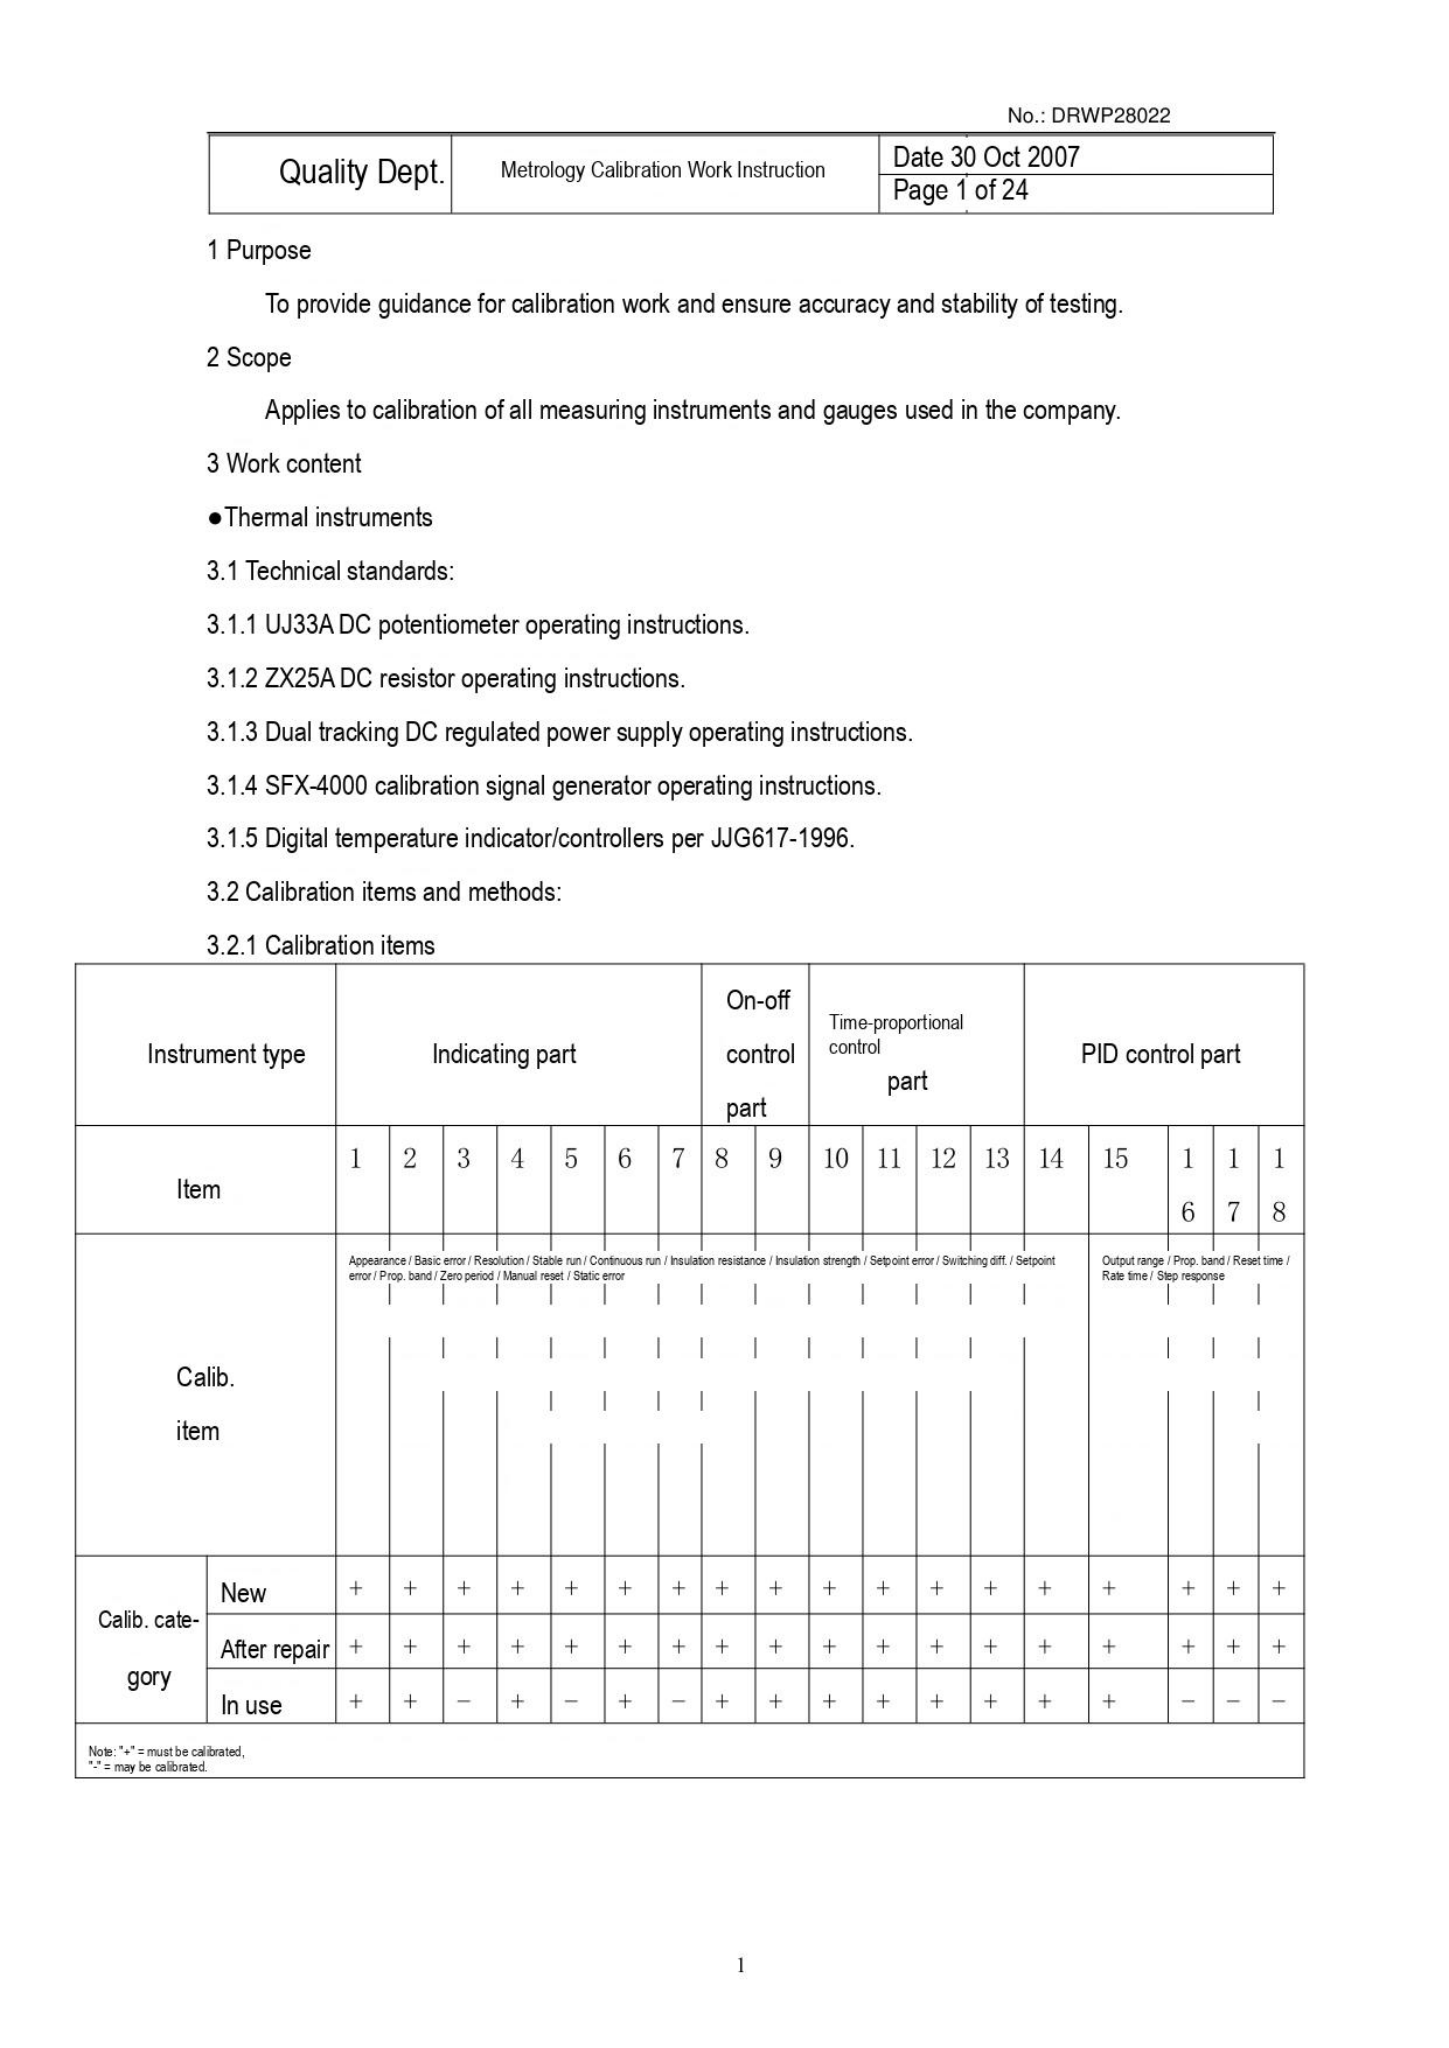No.: DRWP28022

| Quality Dept. | Metrology Calibration Work Instruction | Date 30 Oct 2007 |
|---|---|---|
| | | Page 1 of 24 |

1 Purpose

To provide guidance for calibration work and ensure accuracy and stability of testing.

2 Scope

Applies to calibration of all measuring instruments and gauges used in the company.

3 Work content

●Thermal instruments

3.1 Technical standards:

3.1.1 UJ33A DC potentiometer operating instructions.

3.1.2 ZX25A DC resistor operating instructions.

3.1.3 Dual tracking DC regulated power supply operating instructions.

3.1.4 SFX-4000 calibration signal generator operating instructions.

3.1.5 Digital temperature indicator/controllers per JJG617-1996.

3.2 Calibration items and methods:

3.2.1 Calibration items

| Instrument type | | Indicating part | | | | | | | On-off control part | | Time-proportional control part | | | | PID control part | | | | |
|---|---|---|---|---|---|---|---|---|---|---|---|---|---|---|---|---|---|---|---|
| Item | | 1 | 2 | 3 | 4 | 5 | 6 | 7 | 8 | 9 | 10 | 11 | 12 | 13 | 14 | 15 | 16 | 17 | 18 |
| Calib. item | | Appearance / Basic error / Resolution / Stable run / Continuous run / Insulation resistance / Insulation strength / Setpoint error / Switching diff. / Setpoint error / Prop. band / Zero period / Manual reset / Static error | | | | | | | | | | | | | | Output range / Prop. band / Reset time / Rate time / Step response | | | |
| Calib. category | New | + | + | + | + | + | + | + | + | + | + | + | + | + | + | + | + | + | + |
| | After repair | + | + | + | + | + | + | + | + | + | + | + | + | + | + | + | + | + | + |
| | In use | + | + | − | + | − | + | − | + | + | + | + | + | + | + | + | − | − | − |
| Note: "+" = must be calibrated, "-" = may be calibrated. | | | | | | | | | | | | | | | | | | | |

1
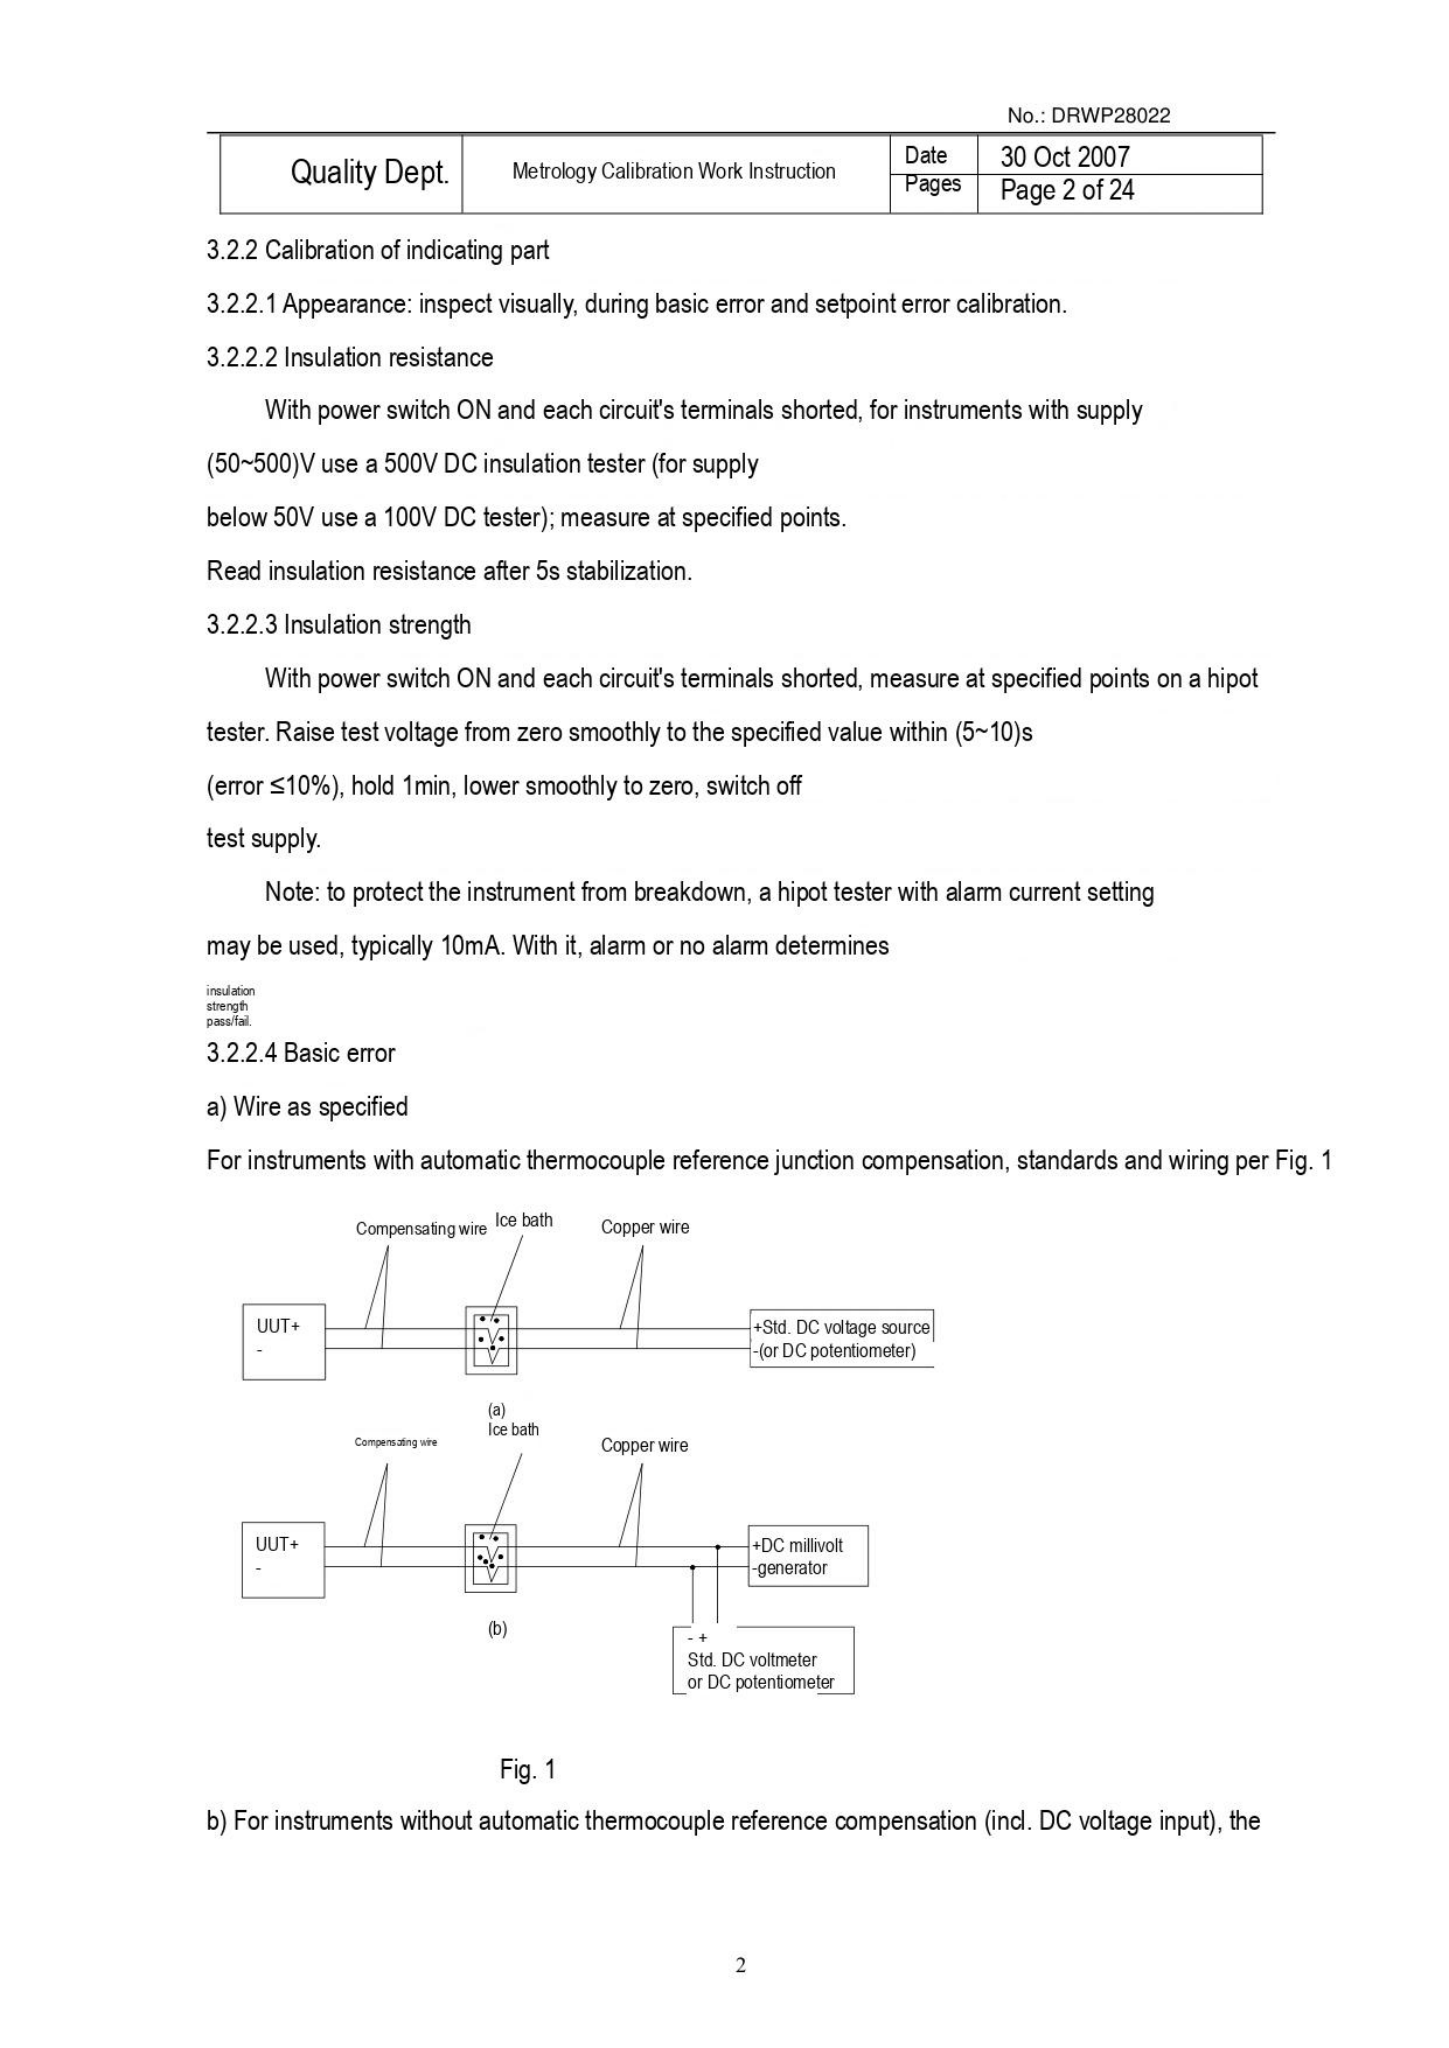No.: DRWP28022

| Quality Dept. | Metrology Calibration Work Instruction | Date | 30 Oct 2007 |
|---|---|---|---|
| | | Pages | Page 2 of 24 |

3.2.2 Calibration of indicating part

3.2.2.1 Appearance: inspect visually, during basic error and setpoint error calibration.

3.2.2.2 Insulation resistance

With power switch ON and each circuit's terminals shorted, for instruments with supply (50~500)V use a 500V DC insulation tester (for supply below 50V use a 100V DC tester); measure at specified points. Read insulation resistance after 5s stabilization.

3.2.2.3 Insulation strength

With power switch ON and each circuit's terminals shorted, measure at specified points on a hipot tester. Raise test voltage from zero smoothly to the specified value within (5~10)s (error ≤10%), hold 1min, lower smoothly to zero, switch off test supply.

Note: to protect the instrument from breakdown, a hipot tester with alarm current setting may be used, typically 10mA. With it, alarm or no alarm determines insulation strength pass/fail.

3.2.2.4 Basic error

a) Wire as specified

For instruments with automatic thermocouple reference junction compensation, standards and wiring per Fig. 1

Compensating wire Ice bath Copper wire

UUT+
-

+Std. DC voltage source
-(or DC potentiometer)

(a)

Ice bath

Compensating wire

Copper wire

UUT+
-

+DC millivolt
-generator

- +
Std. DC voltmeter
or DC potentiometer

(b)

Fig. 1

b) For instruments without automatic thermocouple reference compensation (incl. DC voltage input), the

2
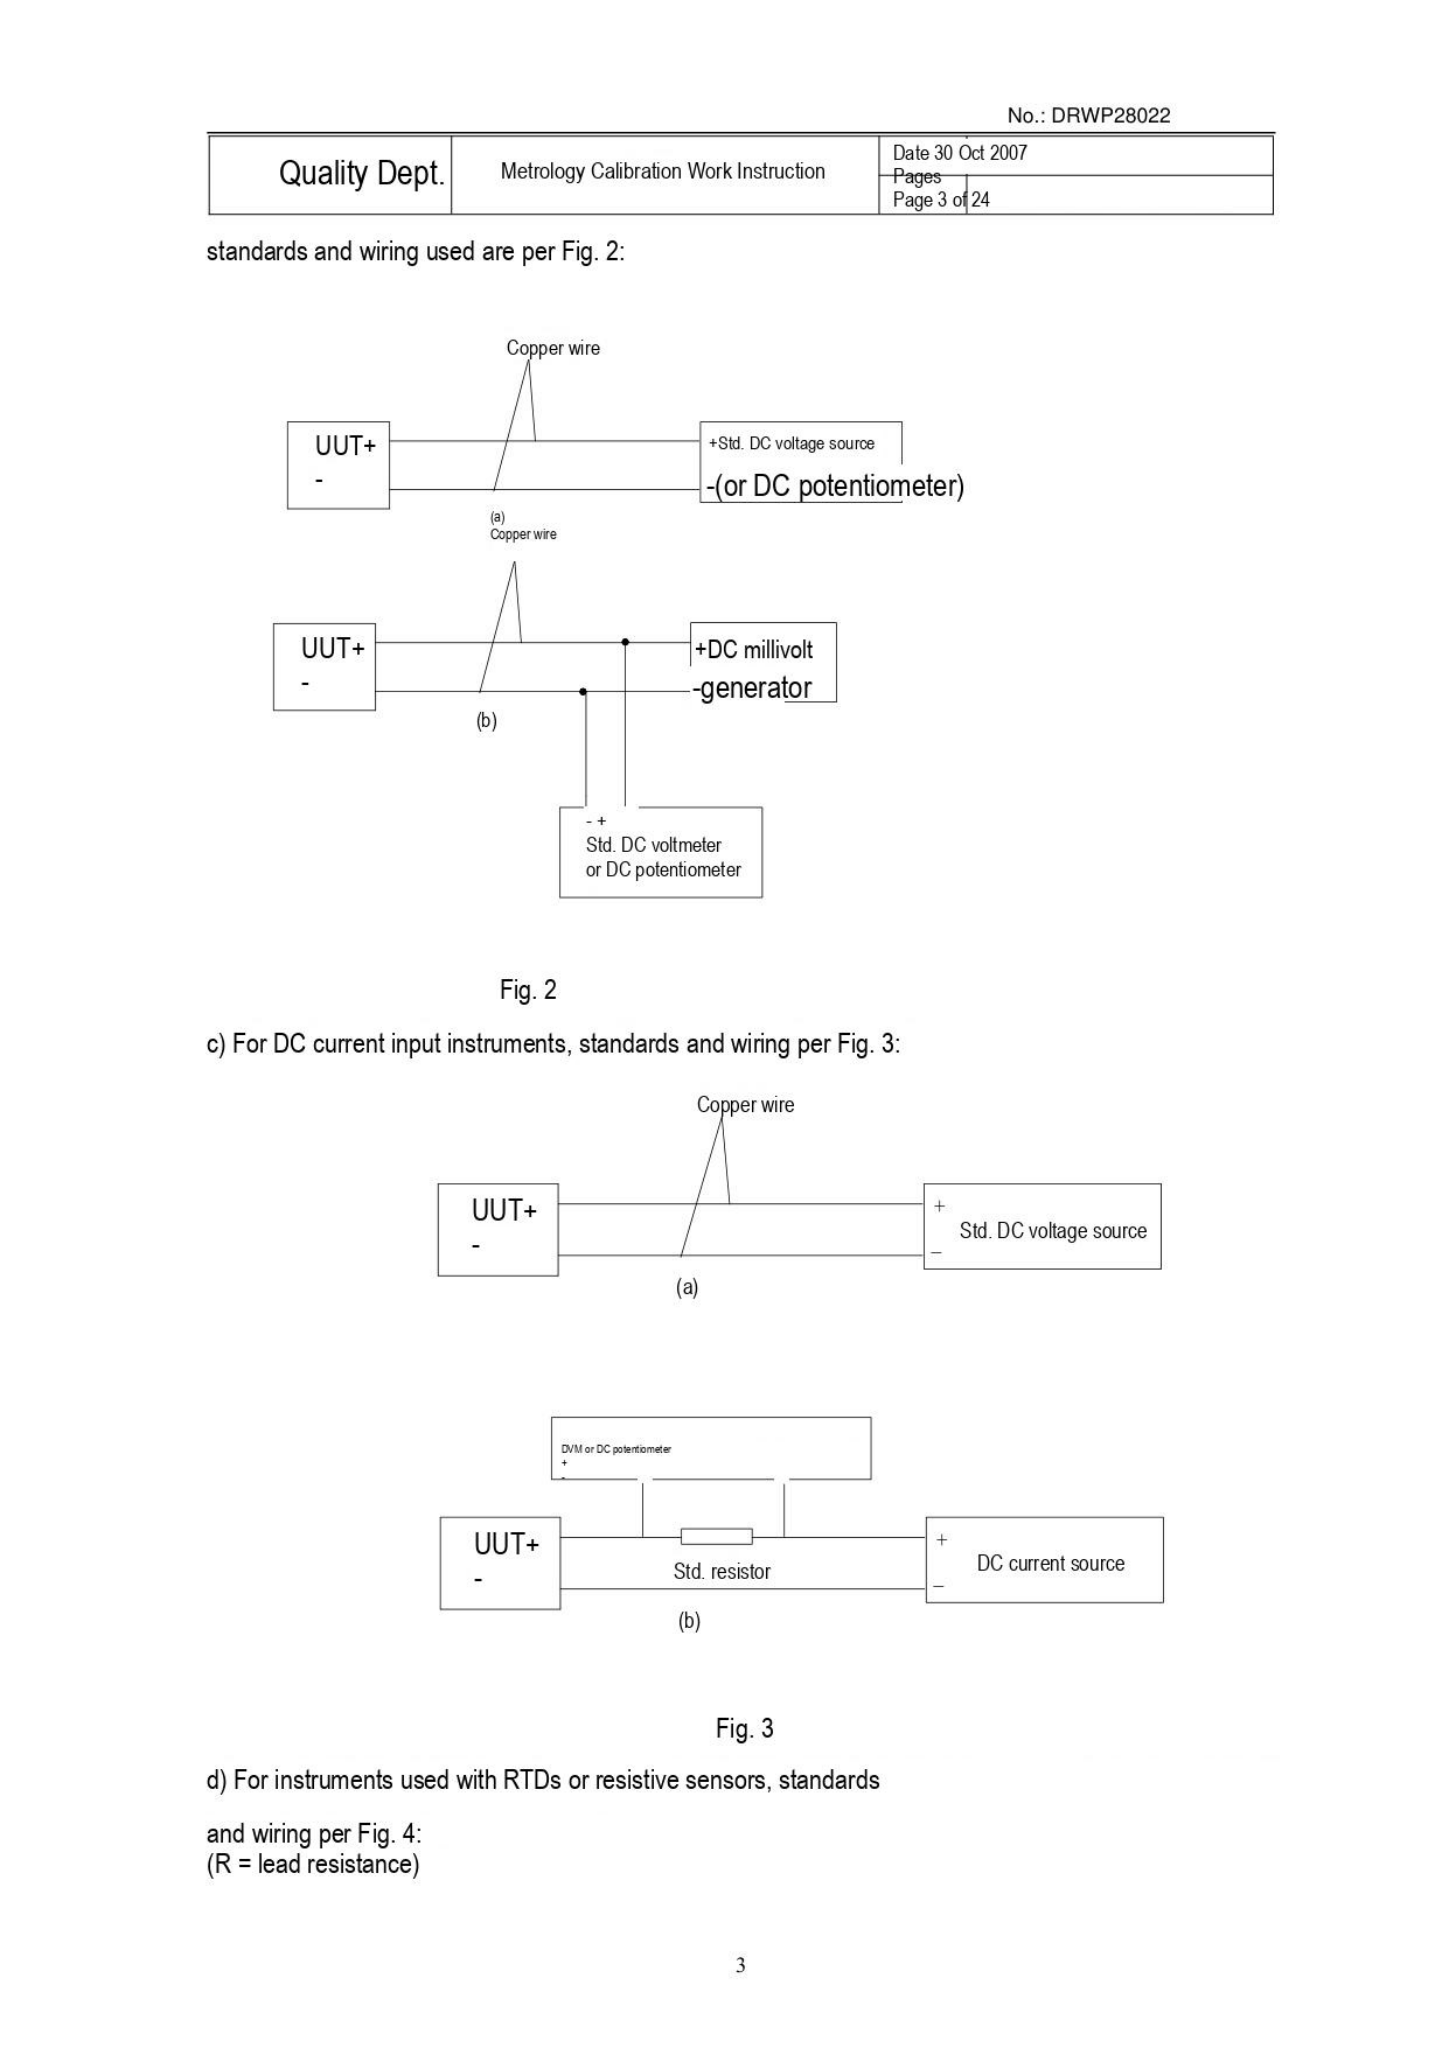No.: DRWP28022

| Quality Dept. | Metrology Calibration Work Instruction | Date 30 Oct 2007<br>Pages<br>Page 3 of 24 |
|---|---|---|

standards and wiring used are per Fig. 2:

Copper wire

UUT+
-

+Std. DC voltage source
-(or DC potentiometer)

(a)
Copper wire

UUT+
-

+DC millivolt
-generator

(b)

- +
Std. DC voltmeter
or DC potentiometer

Fig. 2

c) For DC current input instruments, standards and wiring per Fig. 3:

Copper wire

UUT+
-

+
Std. DC voltage source
–

(a)

DVM or DC potentiometer
+
-

UUT+
-

Std. resistor

+
DC current source
–

(b)

Fig. 3

d) For instruments used with RTDs or resistive sensors, standards

and wiring per Fig. 4:
(R = lead resistance)

3
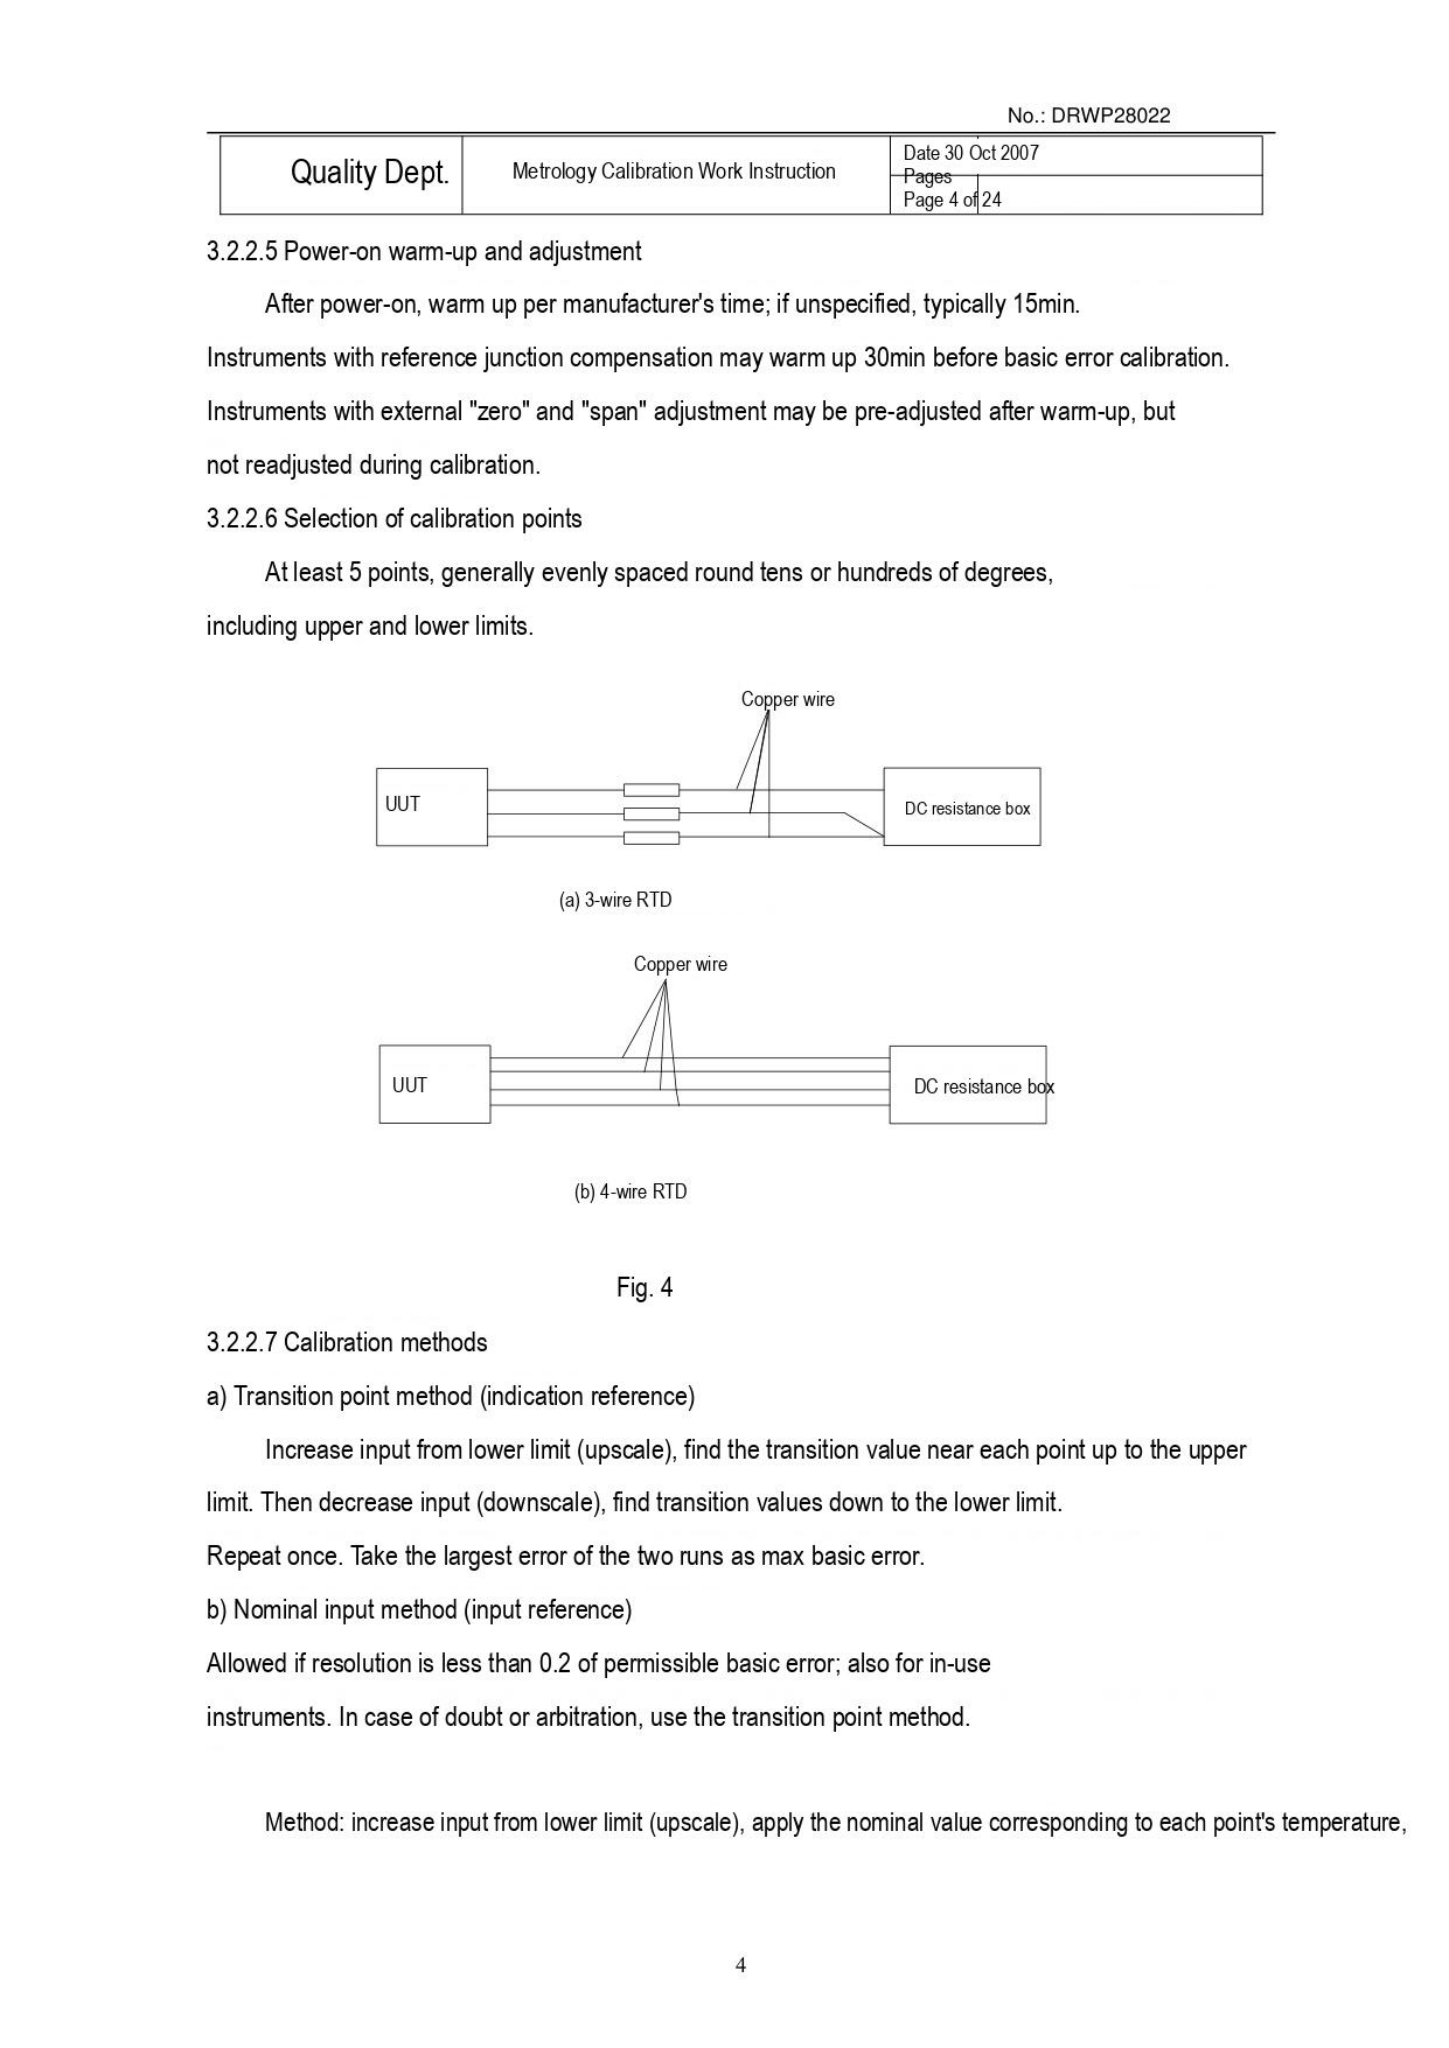No.: DRWP28022

| Quality Dept. | Metrology Calibration Work Instruction | Date 30 Oct 2007<br>Pages<br>Page 4 of 24 |
|---|---|---|

3.2.2.5 Power-on warm-up and adjustment

After power-on, warm up per manufacturer's time; if unspecified, typically 15min. Instruments with reference junction compensation may warm up 30min before basic error calibration. Instruments with external "zero" and "span" adjustment may be pre-adjusted after warm-up, but not readjusted during calibration.

3.2.2.6 Selection of calibration points

At least 5 points, generally evenly spaced round tens or hundreds of degrees, including upper and lower limits.

Copper wire

UUT

DC resistance box

(a) 3-wire RTD

Copper wire

UUT

DC resistance box

(b) 4-wire RTD

Fig. 4

3.2.2.7 Calibration methods

a) Transition point method (indication reference)

Increase input from lower limit (upscale), find the transition value near each point up to the upper limit. Then decrease input (downscale), find transition values down to the lower limit. Repeat once. Take the largest error of the two runs as max basic error.

b) Nominal input method (input reference)

Allowed if resolution is less than 0.2 of permissible basic error; also for in-use instruments. In case of doubt or arbitration, use the transition point method.

Method: increase input from lower limit (upscale), apply the nominal value corresponding to each point's temperature,

4
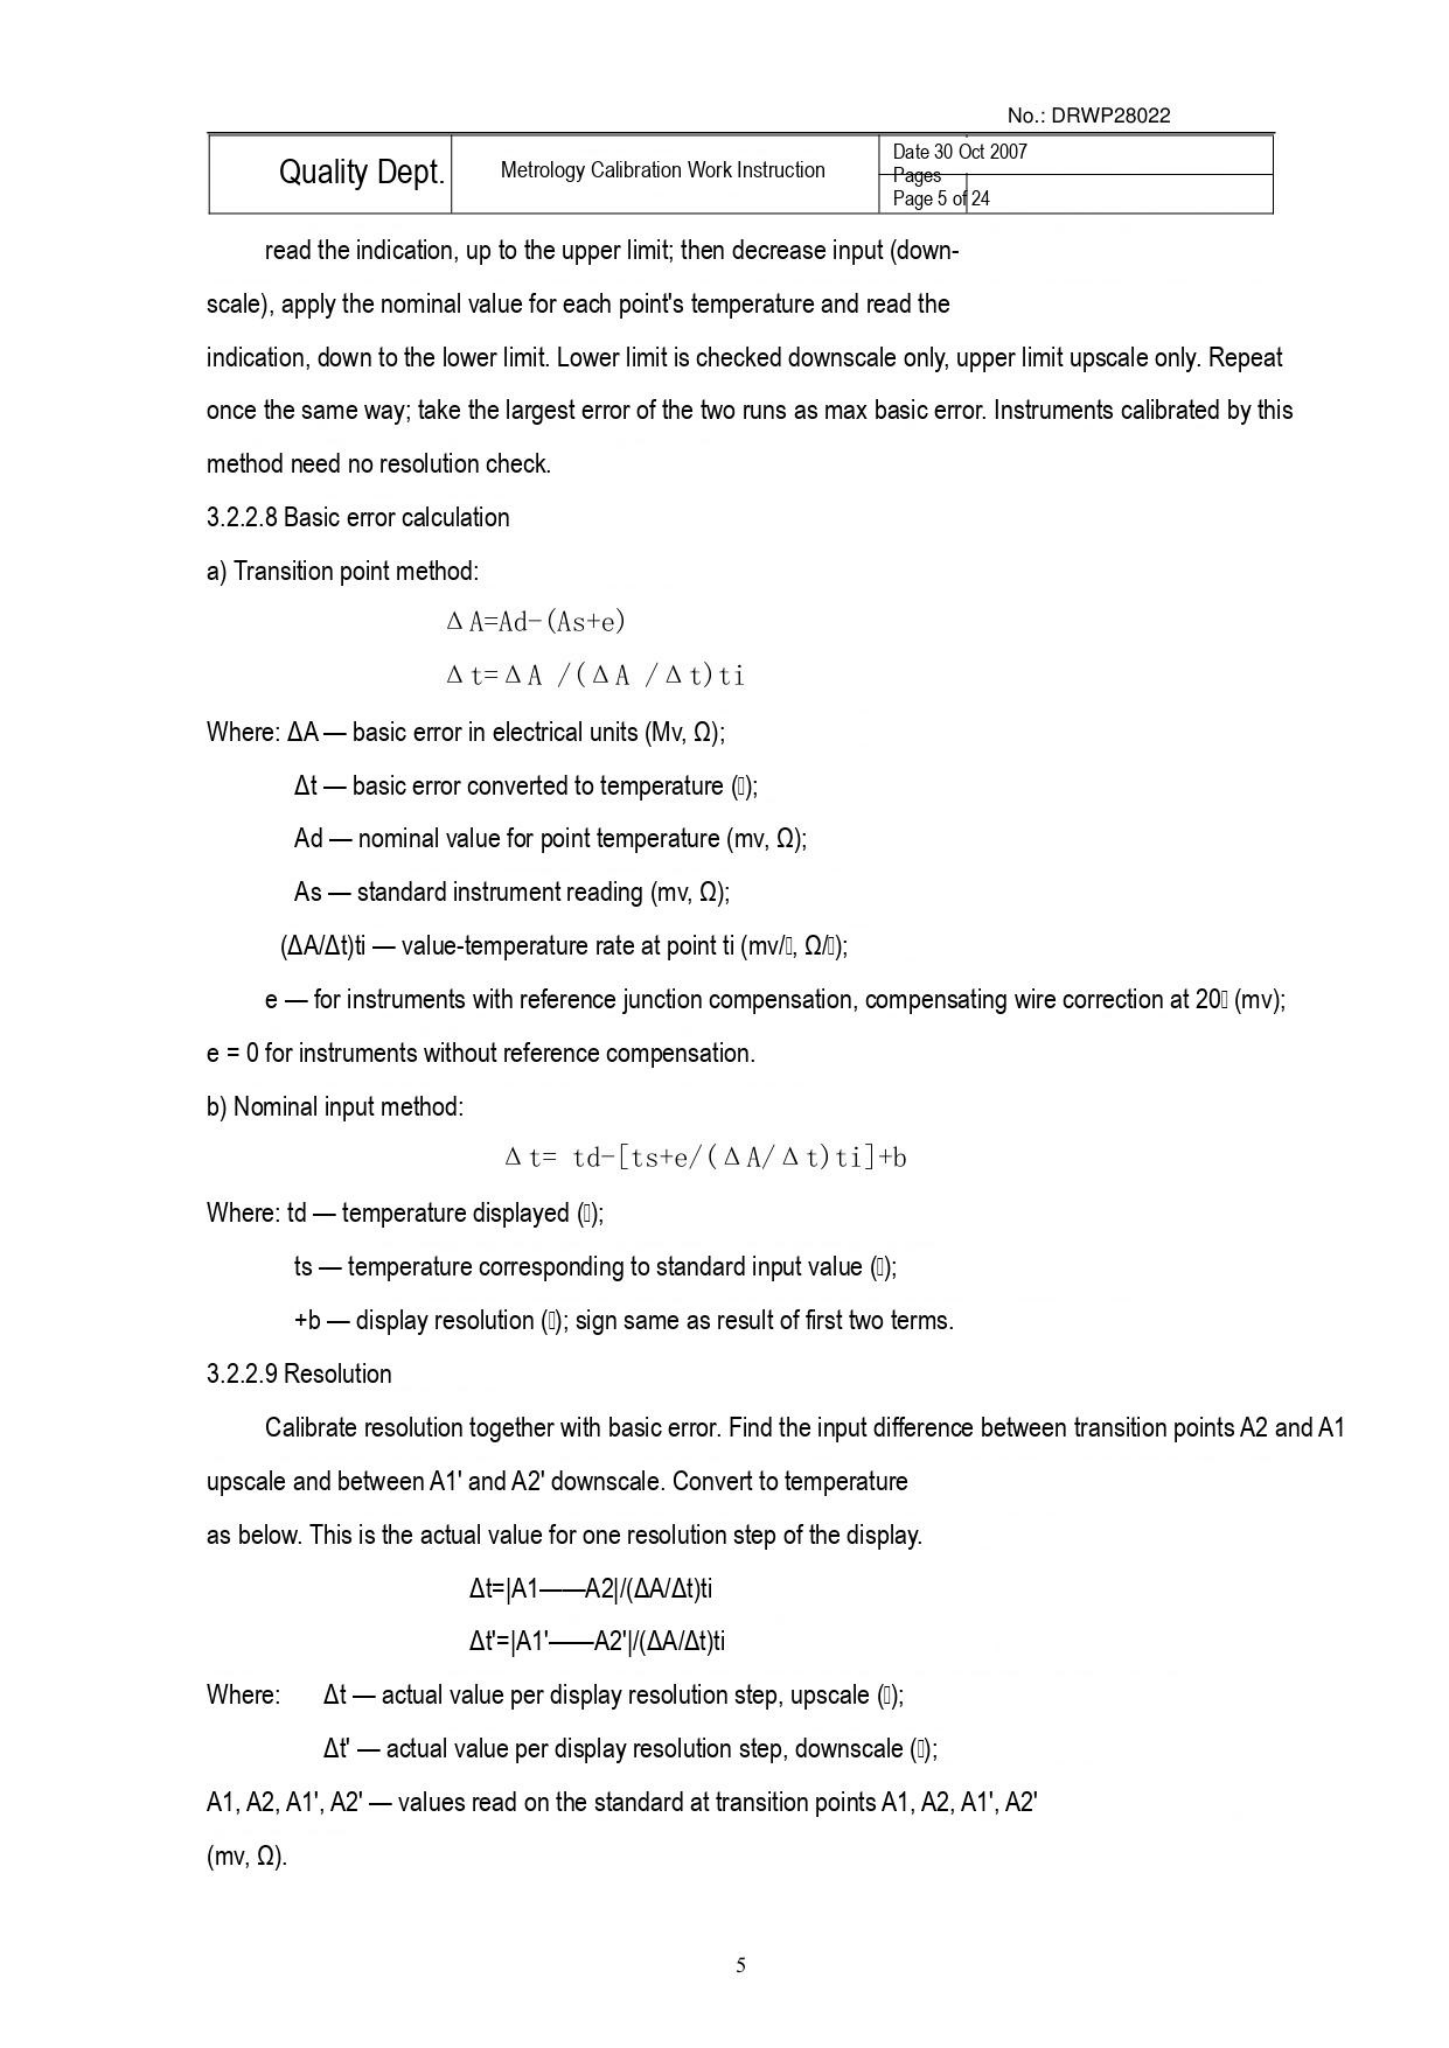No.: DRWP28022

| Quality Dept. | Metrology Calibration Work Instruction | Date 30 Oct 2007<br>Pages<br>Page 5 of 24 |
|---|---|---|

read the indication, up to the upper limit; then decrease input (down-scale), apply the nominal value for each point's temperature and read the indication, down to the lower limit. Lower limit is checked downscale only, upper limit upscale only. Repeat once the same way; take the largest error of the two runs as max basic error. Instruments calibrated by this method need no resolution check.

3.2.2.8 Basic error calculation

a) Transition point method:

ΔA=Ad-(As+e)

Δt=ΔA /(ΔA /Δt)ti

Where: ΔA — basic error in electrical units (Mv, Ω);

Δt — basic error converted to temperature ();

Ad — nominal value for point temperature (mv, Ω);

As — standard instrument reading (mv, Ω);

(ΔA/Δt)ti — value-temperature rate at point ti (mv/, Ω/);

e — for instruments with reference junction compensation, compensating wire correction at 20 (mv); e = 0 for instruments without reference compensation.

b) Nominal input method:

Δt= td-[ts+e/(ΔA/Δt)ti]+b

Where: td — temperature displayed ();

ts — temperature corresponding to standard input value ();

+b — display resolution (); sign same as result of first two terms.

3.2.2.9 Resolution

Calibrate resolution together with basic error. Find the input difference between transition points A2 and A1 upscale and between A1' and A2' downscale. Convert to temperature as below. This is the actual value for one resolution step of the display.

Δt=|A1——A2|/(ΔA/Δt)ti

Δt'=|A1'——A2'|/(ΔA/Δt)ti

Where: Δt — actual value per display resolution step, upscale ();

Δt' — actual value per display resolution step, downscale ();

A1, A2, A1', A2' — values read on the standard at transition points A1, A2, A1', A2' (mv, Ω).

5
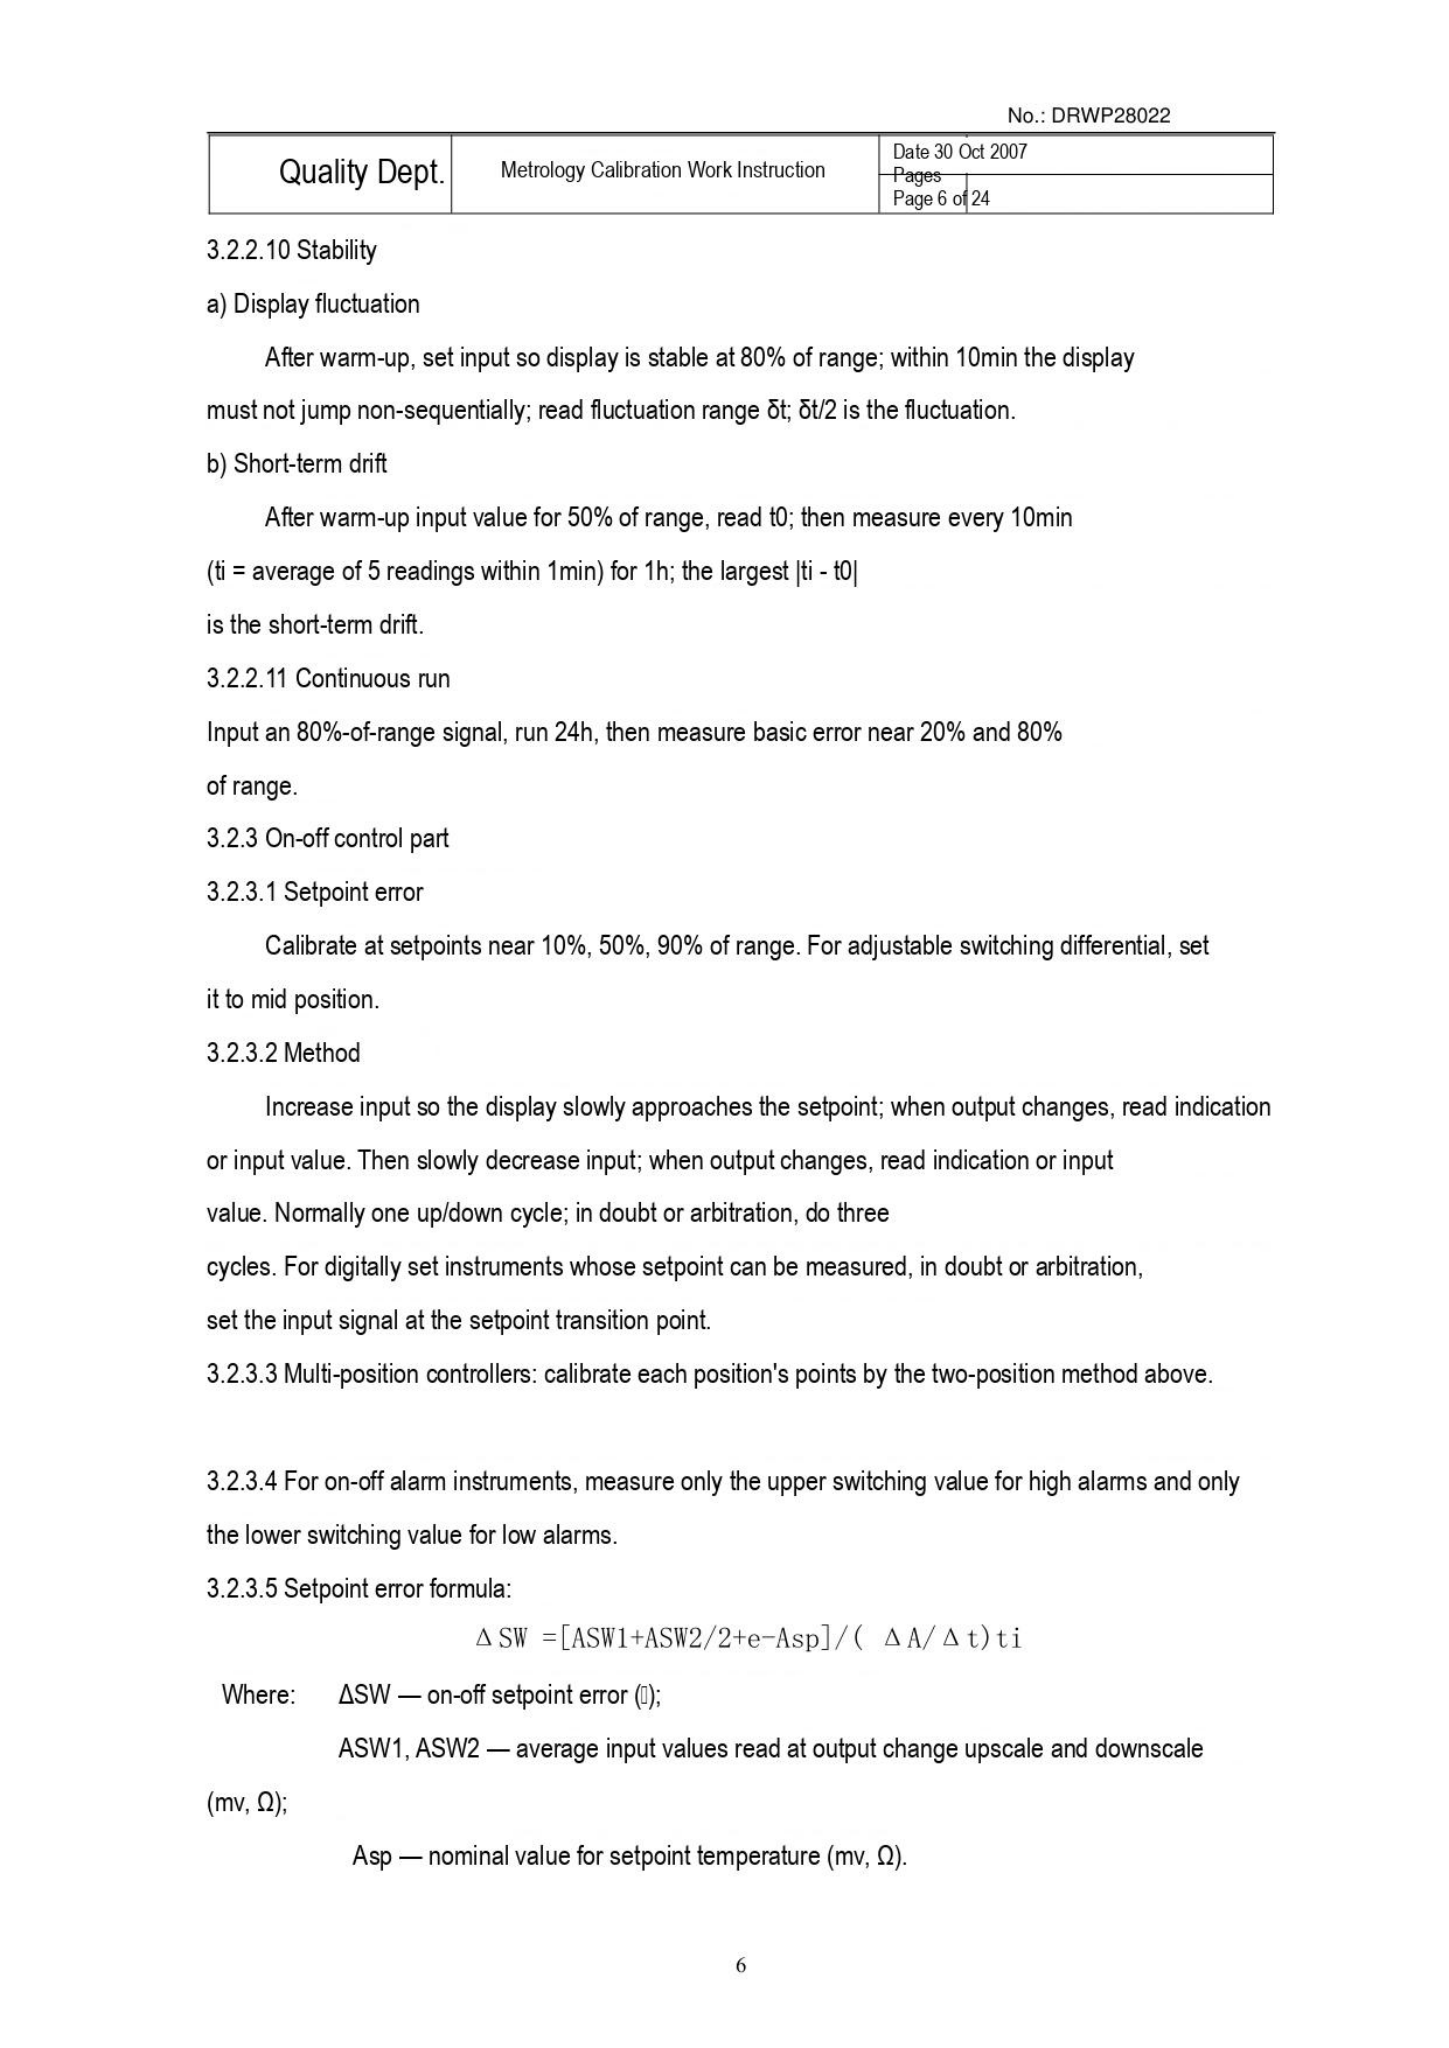No.: DRWP28022

| Quality Dept. | Metrology Calibration Work Instruction | Date 30 Oct 2007<br>Pages<br>Page 6 of 24 |
|---|---|---|

3.2.2.10 Stability

a) Display fluctuation

After warm-up, set input so display is stable at 80% of range; within 10min the display must not jump non-sequentially; read fluctuation range δt; δt/2 is the fluctuation.

b) Short-term drift

After warm-up input value for 50% of range, read t0; then measure every 10min (ti = average of 5 readings within 1min) for 1h; the largest |ti - t0| is the short-term drift.

3.2.2.11 Continuous run

Input an 80%-of-range signal, run 24h, then measure basic error near 20% and 80% of range.

3.2.3 On-off control part

3.2.3.1 Setpoint error

Calibrate at setpoints near 10%, 50%, 90% of range. For adjustable switching differential, set it to mid position.

3.2.3.2 Method

Increase input so the display slowly approaches the setpoint; when output changes, read indication or input value. Then slowly decrease input; when output changes, read indication or input value. Normally one up/down cycle; in doubt or arbitration, do three cycles. For digitally set instruments whose setpoint can be measured, in doubt or arbitration, set the input signal at the setpoint transition point.

3.2.3.3 Multi-position controllers: calibrate each position's points by the two-position method above.

3.2.3.4 For on-off alarm instruments, measure only the upper switching value for high alarms and only the lower switching value for low alarms.

3.2.3.5 Setpoint error formula:

ΔSW =[ASW1+ASW2/2+e−Asp]/( ΔA/Δt)ti

Where: ΔSW — on-off setpoint error ();

ASW1, ASW2 — average input values read at output change upscale and downscale (mv, Ω);

Asp — nominal value for setpoint temperature (mv, Ω).

6
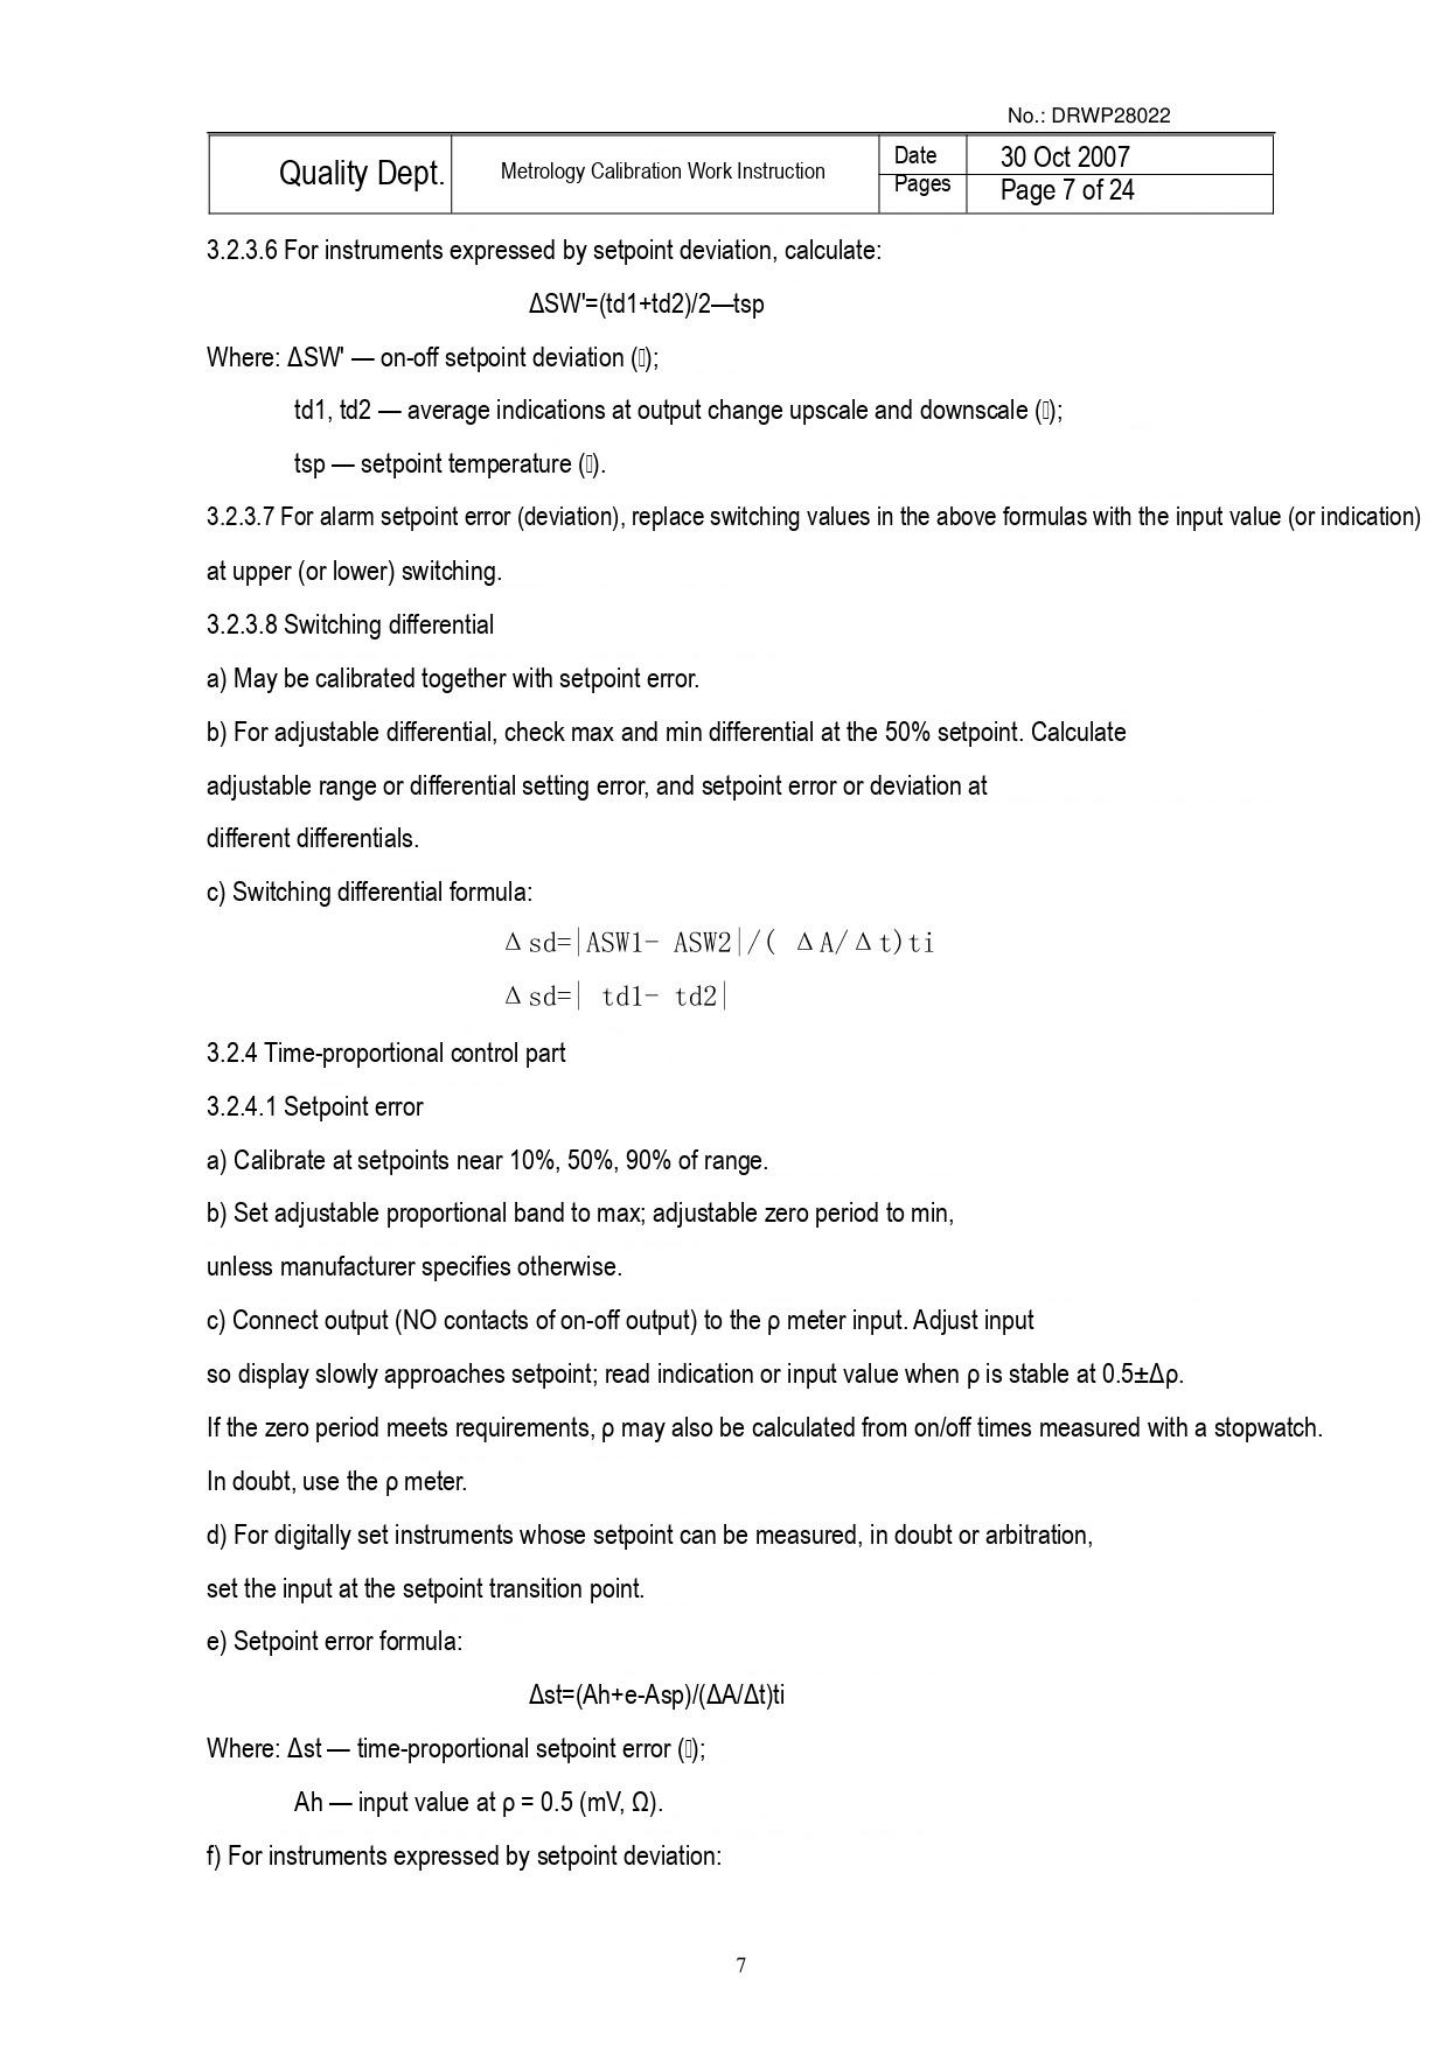No.: DRWP28022

| Quality Dept. | Metrology Calibration Work Instruction | Date | 30 Oct 2007 |
|---|---|---|---|
| | | Pages | Page 7 of 24 |

3.2.3.6 For instruments expressed by setpoint deviation, calculate:

ΔSW'=(td1+td2)/2—tsp

Where: ΔSW' — on-off setpoint deviation ();

td1, td2 — average indications at output change upscale and downscale ();

tsp — setpoint temperature ().

3.2.3.7 For alarm setpoint error (deviation), replace switching values in the above formulas with the input value (or indication) at upper (or lower) switching.

3.2.3.8 Switching differential

a) May be calibrated together with setpoint error.

b) For adjustable differential, check max and min differential at the 50% setpoint. Calculate adjustable range or differential setting error, and setpoint error or deviation at different differentials.

c) Switching differential formula:

Δ sd=|ASW1- ASW2|/( ΔA/Δt)ti

Δ sd=| td1- td2|

3.2.4 Time-proportional control part

3.2.4.1 Setpoint error

a) Calibrate at setpoints near 10%, 50%, 90% of range.

b) Set adjustable proportional band to max; adjustable zero period to min, unless manufacturer specifies otherwise.

c) Connect output (NO contacts of on-off output) to the ρ meter input. Adjust input so display slowly approaches setpoint; read indication or input value when ρ is stable at 0.5±Δρ. If the zero period meets requirements, ρ may also be calculated from on/off times measured with a stopwatch. In doubt, use the ρ meter.

d) For digitally set instruments whose setpoint can be measured, in doubt or arbitration, set the input at the setpoint transition point.

e) Setpoint error formula:

Δst=(Ah+e-Asp)/(ΔA/Δt)ti

Where: Δst — time-proportional setpoint error ();

Ah — input value at ρ = 0.5 (mV, Ω).

f) For instruments expressed by setpoint deviation:

7